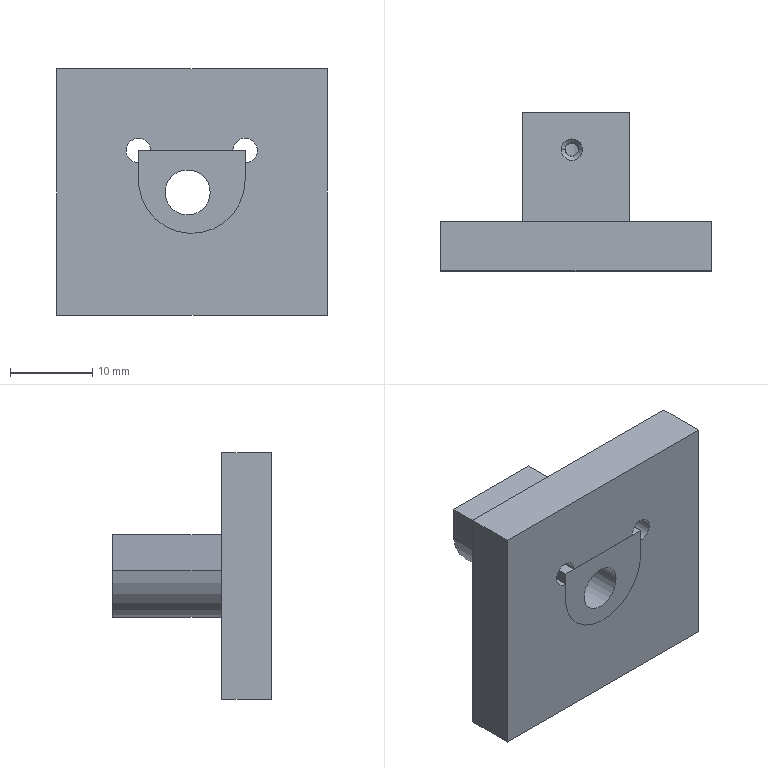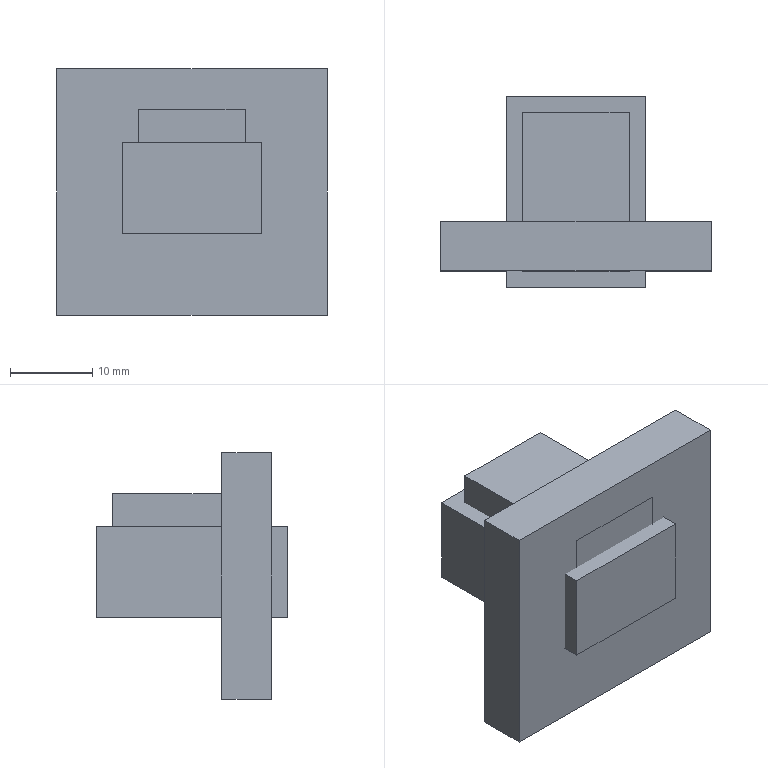CAM job | NX | 3+2 milling, drilling | part box 32.951 x 19.3 x 30.1 mm | stock box 32.951 x 23.3 x 30.1 mm
Tools:
number,name,description,diameter,corner_radius,flute_length,length,flutes
6,D6,Milling Tool-5 Parameters,6.0,0.0,50.0,75.0,2
1,D63,Milling Tool-5 Parameters,63.0,0.0,50.0,75.0,2
7,D6A45,Milling Tool-5 Parameters,6.0,0.0,50.0,75.0,2
16,1.6ZT,Drilling Tool,1.6,0.0,35.0,50.0,2
15,5.5ZT,Drilling Tool,5.5,0.0,35.0,50.0,2
2,D2,Milling Tool-5 Parameters,2.0,0.0,50.0,75.0,2
Operations:
program,operation,operation_type,tool,method,geometry_group,spindle_rpm,surface_speed,feed_per_tooth,feed_cut,feed_plunge,cut_length_mm,path_length_mm,cut_time_min,machine_time_min
11,FLOOR_WALL_COPY,VolumeBased25DMillingOperation,D63,METHOD,C,6500.0,122.0,0.1154,1500.0,100.0,87.907,141.907,0.0586,0.064
11,DRILLING_COPY_1,Operation,D6A45,METHOD,C,5000.0,94.0,0.025,250.0,0.0,4.3,68.6,0.0172,0.0236
11,DRILLING_COPY_1_COPY,Operation,5.5ZT,METHOD,C,2000.0,34.0,0.05,200.0,0.0,25.452,110.905,0.1273,0.1358
11,ZLEVEL_PROFILE_COPY_1,ZLevelMilling,D6,METHOD,C,9500.0,179.0,0.1316,2500.0,1000.0,2411.868,2488.168,0.9876,0.9952
11,ZLEVEL_PROFILE_COPY_COPY,ZLevelMilling,D6,METHOD,C,9500.0,179.0,0.0684,1300.0,1000.0,131.343,305.259,0.1024,0.1198
11,PLANAR_MILL_COPY,PlanarMilling,D6A45,METHOD,C,9500.0,179.0,0.0658,1250.0,100.0,20.864,79.864,0.0167,0.0226
11,PLANAR_MILL_COPY_COPY,PlanarMilling,D6A45,METHOD,C,9500.0,179.0,0.0658,1250.0,100.0,53.132,112.132,0.0425,0.0484
22,FLOOR_WALL_COPY_COPY,VolumeBased25DMillingOperation,D63,METHOD,B,6500.0,122.0,0.1154,1500.0,100.0,425.5,991.901,0.2837,0.3403
22,PLANAR_MILL_COPY_COPY_COPY,PlanarMilling,D6A45,METHOD,B,9500.0,179.0,0.0658,1250.0,100.0,67.388,190.278,0.0539,0.0662
33,DRILLING,Operation,D6A45,METHOD,A,5000.0,94.0,0.025,250.0,0.0,8.6,91.275,0.0344,0.0427
33,DRILLING_COPY,Operation,1.6ZT,METHOD,A,2000.0,10.0,0.025,100.0,0.0,14.899,103.873,0.149,0.1579
33,PLANAR_MILL,PlanarMilling,D6A45,METHOD,A,9500.0,179.0,0.0658,1250.0,100.0,77.029,136.029,0.0616,0.0675
4,PLANAR_MILL_1,PlanarMilling,D2,METHOD,D,9500.0,59.0,0.0632,1200.0,100.0,5372.324,5609.293,4.477,4.501